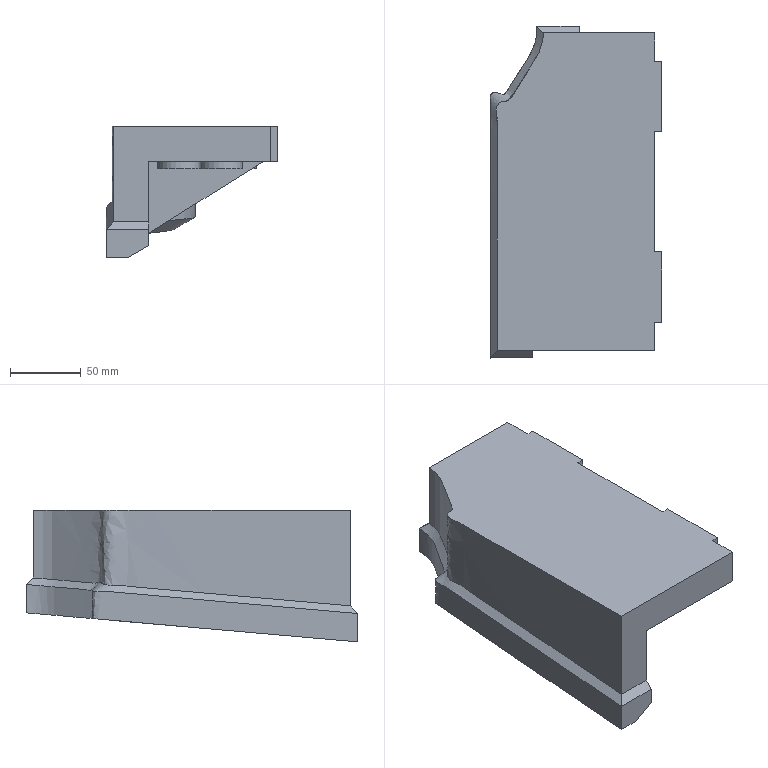Part | NX | features solid 2 | 1 solid | 38 faces | box 121.925 x 235 x 93.265 mm | volume 1020606 mm3 | plane 27 | spline 6 | cylinder 5 | commonest cylinder face diameters 30 x5